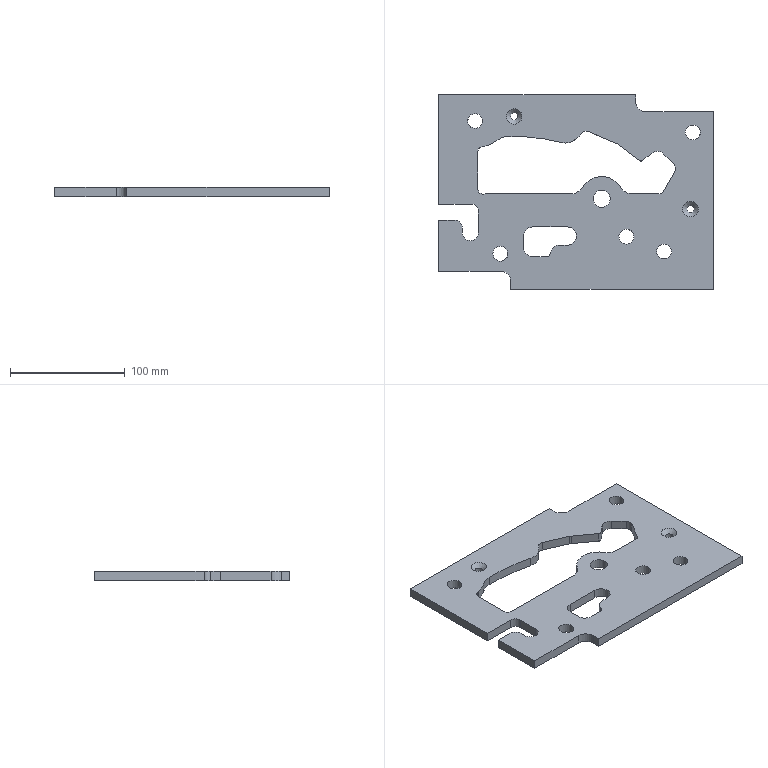Part | STEP file | gslz 2016.10.28-13_id142_x_t | 1 solid | 64 faces | box 240 x 170 x 8 mm | volume 233843 mm3 | cylinder 35 | plane 27 | cone 2 | commonest cylinder face diameters 10 x6 13 x5 16 x4 14 x3 6.5 x2 18 x2